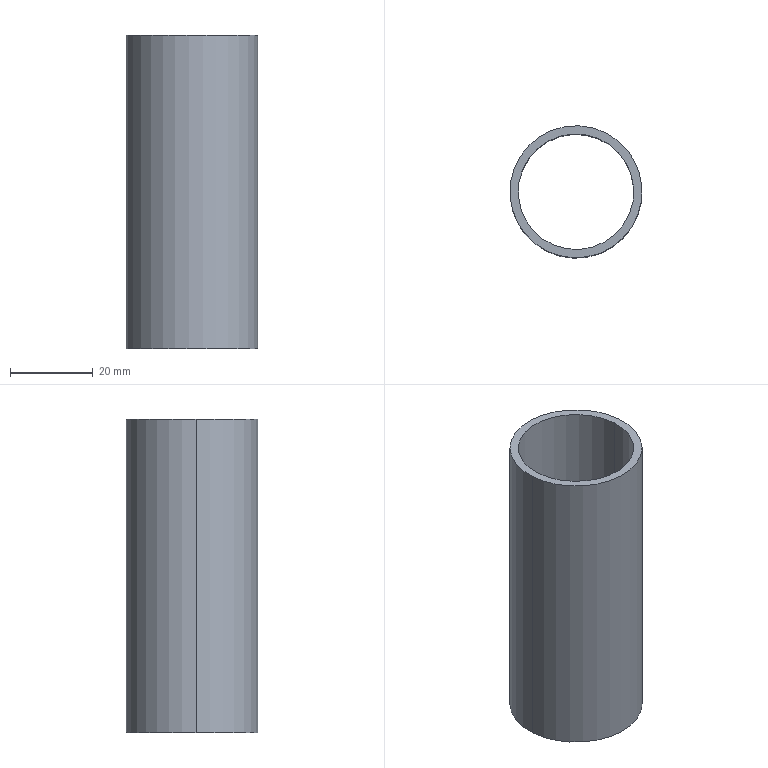Part | NX | features 0018 2 | 1 solid | 6 faces | box 32 x 32 x 76 mm | volume 14326 mm3 | cylinder 4 | plane 2 | commonest cylinder face diameters 28 x2 32 x2
STEP:
#1=CARTESIAN_POINT('',(-66.026,25.859,-286.129));
#2=VERTEX_POINT('',#1);
#3=CARTESIAN_POINT('',(-93.974,24.141,-286.129));
#4=VERTEX_POINT('',#3);
#5=CARTESIAN_POINT('',(-80.,25.,-286.129));
#6=DIRECTION('',(0.,0.,1.));
#7=DIRECTION('',(0.9981,0.06136,0.));
#8=AXIS2_PLACEMENT_3D('',#5,#6,#7);
#9=CIRCLE('',#8,14.);
#10=EDGE_CURVE('',#2,#4,#9,.T.);
#11=ORIENTED_EDGE('',*,*,#10,.F.);
#12=CARTESIAN_POINT('',(-66.026,25.859,-210.129));
#13=VERTEX_POINT('',#12);
#14=CARTESIAN_POINT('',(-66.026,25.859,-210.129));
#15=DIRECTION('',(0.,0.,-1.));
#16=VECTOR('',#15,1000.);
#17=LINE('',#14,#16);
#18=EDGE_CURVE('',#13,#2,#17,.T.);
#19=ORIENTED_EDGE('',*,*,#18,.F.);
#20=CARTESIAN_POINT('',(-93.974,24.141,-210.129));
#21=VERTEX_POINT('',#20);
#22=CARTESIAN_POINT('',(-80.,25.,-210.129));
#23=DIRECTION('',(0.,0.,-1.));
#24=DIRECTION('',(-0.9981,-0.06136,0.));
#25=AXIS2_PLACEMENT_3D('',#22,#23,#24);
#26=CIRCLE('',#25,14.);
#27=EDGE_CURVE('',#21,#13,#26,.T.);
#28=ORIENTED_EDGE('',*,*,#27,.F.);
#29=CARTESIAN_POINT('',(-93.974,24.141,-210.129));
#30=DIRECTION('',(0.,0.,-1.));
#31=VECTOR('',#30,1000.);
#32=LINE('',#29,#31);
#33=EDGE_CURVE('',#4,#21,#32,.F.);
#34=ORIENTED_EDGE('',*,*,#33,.F.);
#35=EDGE_LOOP('',(#11,#19,#28,#34));
#36=FACE_BOUND('',#35,.T.);
#37=CARTESIAN_POINT('',(-80.,25.,-286.129));
#38=DIRECTION('',(0.,0.,1.));
#39=DIRECTION('',(0.9981,0.06136,0.));
#40=AXIS2_PLACEMENT_3D('',#37,#38,#39);
#41=CYLINDRICAL_SURFACE('',#40,14.);
#42=ADVANCED_FACE('',(#36),#41,.F.);
#43=ORIENTED_EDGE('',*,*,#27,.T.);
#44=CARTESIAN_POINT('',(-80.,25.,-210.129));
#45=DIRECTION('',(0.,0.,-1.));
#46=DIRECTION('',(0.9981,0.06136,0.));
#47=AXIS2_PLACEMENT_3D('',#44,#45,#46);
#48=CIRCLE('',#47,14.);
#49=EDGE_CURVE('',#13,#21,#48,.T.);
#50=ORIENTED_EDGE('',*,*,#49,.T.);
#51=EDGE_LOOP('',(#43,#50));
#52=FACE_BOUND('',#51,.T.);
#53=CARTESIAN_POINT('',(-64.03,25.982,-210.129));
#54=VERTEX_POINT('',#53);
#55=CARTESIAN_POINT('',(-95.97,24.018,-210.129));
#56=VERTEX_POINT('',#55);
#57=CARTESIAN_POINT('',(-80.,25.,-210.129));
#58=DIRECTION('',(0.,0.,1.));
#59=DIRECTION('',(0.9981,0.06136,0.));
#60=AXIS2_PLACEMENT_3D('',#57,#58,#59);
#61=CIRCLE('',#60,16.);
#62=EDGE_CURVE('',#54,#56,#61,.T.);
#63=ORIENTED_EDGE('',*,*,#62,.T.);
#64=CARTESIAN_POINT('',(-80.,25.,-210.129));
#65=DIRECTION('',(0.,0.,1.));
#66=DIRECTION('',(-0.9981,-0.06136,0.));
#67=AXIS2_PLACEMENT_3D('',#64,#65,#66);
#68=CIRCLE('',#67,16.);
#69=EDGE_CURVE('',#56,#54,#68,.T.);
#70=ORIENTED_EDGE('',*,*,#69,.T.);
#71=EDGE_LOOP('',(#63,#70));
#72=FACE_BOUND('',#71,.T.);
#73=CARTESIAN_POINT('',(-80.,25.,-210.129));
#74=DIRECTION('',(0.,0.,-1.));
#75=DIRECTION('',(-0.9981,-0.06136,0.));
#76=AXIS2_PLACEMENT_3D('',#73,#74,#75);
#77=PLANE('',#76);
#78=ADVANCED_FACE('',(#52,#72),#77,.F.);
#79=CARTESIAN_POINT('',(-95.97,24.018,-286.129));
#80=VERTEX_POINT('',#79);
#81=CARTESIAN_POINT('',(-95.97,24.018,-210.129));
#82=DIRECTION('',(0.,0.,-1.));
#83=VECTOR('',#82,1000.);
#84=LINE('',#81,#83);
#85=EDGE_CURVE('',#56,#80,#84,.T.);
#86=ORIENTED_EDGE('',*,*,#85,.F.);
#87=ORIENTED_EDGE('',*,*,#62,.F.);
#88=CARTESIAN_POINT('',(-64.03,25.982,-286.129));
#89=VERTEX_POINT('',#88);
#90=CARTESIAN_POINT('',(-64.03,25.982,-210.129));
#91=DIRECTION('',(0.,0.,-1.));
#92=VECTOR('',#91,1000.);
#93=LINE('',#90,#92);
#94=EDGE_CURVE('',#89,#54,#93,.F.);
#95=ORIENTED_EDGE('',*,*,#94,.F.);
#96=CARTESIAN_POINT('',(-80.,25.,-286.129));
#97=DIRECTION('',(0.,0.,-1.));
#98=DIRECTION('',(-0.9981,-0.06136,0.));
#99=AXIS2_PLACEMENT_3D('',#96,#97,#98);
#100=CIRCLE('',#99,16.);
#101=EDGE_CURVE('',#80,#89,#100,.T.);
#102=ORIENTED_EDGE('',*,*,#101,.F.);
#103=EDGE_LOOP('',(#86,#87,#95,#102));
#104=FACE_BOUND('',#103,.T.);
#105=CARTESIAN_POINT('',(-80.,25.,-286.129));
#106=DIRECTION('',(0.,0.,1.));
#107=DIRECTION('',(0.9981,0.06136,0.));
#108=AXIS2_PLACEMENT_3D('',#105,#106,#107);
#109=CYLINDRICAL_SURFACE('',#108,16.);
#110=ADVANCED_FACE('',(#104),#109,.T.);
#111=CARTESIAN_POINT('',(-80.,25.,-286.129));
#112=DIRECTION('',(0.,0.,-1.));
#113=DIRECTION('',(0.9981,0.06136,0.));
#114=AXIS2_PLACEMENT_3D('',#111,#112,#113);
#115=CIRCLE('',#114,16.);
#116=EDGE_CURVE('',#89,#80,#115,.T.);
#117=ORIENTED_EDGE('',*,*,#116,.F.);
#118=ORIENTED_EDGE('',*,*,#94,.T.);
#119=ORIENTED_EDGE('',*,*,#69,.F.);
#120=ORIENTED_EDGE('',*,*,#85,.T.);
#121=EDGE_LOOP('',(#117,#118,#119,#120));
#122=FACE_BOUND('',#121,.T.);
#123=CARTESIAN_POINT('',(-80.,25.,-286.129));
#124=DIRECTION('',(0.,0.,1.));
#125=DIRECTION('',(0.9981,0.06136,0.));
#126=AXIS2_PLACEMENT_3D('',#123,#124,#125);
#127=CYLINDRICAL_SURFACE('',#126,16.);
#128=ADVANCED_FACE('',(#122),#127,.T.);
#129=ORIENTED_EDGE('',*,*,#10,.T.);
#130=CARTESIAN_POINT('',(-80.,25.,-286.129));
#131=DIRECTION('',(0.,0.,1.));
#132=DIRECTION('',(-0.9981,-0.06136,0.));
#133=AXIS2_PLACEMENT_3D('',#130,#131,#132);
#134=CIRCLE('',#133,14.);
#135=EDGE_CURVE('',#4,#2,#134,.T.);
#136=ORIENTED_EDGE('',*,*,#135,.T.);
#137=EDGE_LOOP('',(#129,#136));
#138=FACE_BOUND('',#137,.T.);
#139=ORIENTED_EDGE('',*,*,#101,.T.);
#140=ORIENTED_EDGE('',*,*,#116,.T.);
#141=EDGE_LOOP('',(#139,#140));
#142=FACE_BOUND('',#141,.T.);
#143=CARTESIAN_POINT('',(-80.,25.,-286.129));
#144=DIRECTION('',(0.,0.,-1.));
#145=DIRECTION('',(-0.9981,-0.06136,0.));
#146=AXIS2_PLACEMENT_3D('',#143,#144,#145);
#147=PLANE('',#146);
#148=ADVANCED_FACE('',(#138,#142),#147,.T.);
#149=ORIENTED_EDGE('',*,*,#33,.T.);
#150=ORIENTED_EDGE('',*,*,#49,.F.);
#151=ORIENTED_EDGE('',*,*,#18,.T.);
#152=ORIENTED_EDGE('',*,*,#135,.F.);
#153=EDGE_LOOP('',(#149,#150,#151,#152));
#154=FACE_BOUND('',#153,.T.);
#155=CARTESIAN_POINT('',(-80.,25.,-286.129));
#156=DIRECTION('',(0.,0.,1.));
#157=DIRECTION('',(0.9981,0.06136,0.));
#158=AXIS2_PLACEMENT_3D('',#155,#156,#157);
#159=CYLINDRICAL_SURFACE('',#158,14.);
#160=ADVANCED_FACE('',(#154),#159,.F.);
#161=CLOSED_SHELL('',(#42,#78,#110,#128,#148,#160));
#162=MANIFOLD_SOLID_BREP('',#161);
#163=(LENGTH_UNIT()NAMED_UNIT(*)SI_UNIT(.MILLI.,.METRE.));
#164=UNCERTAINTY_MEASURE_WITH_UNIT(LENGTH_MEASURE(0.00001),#163,'','');
#165=(NAMED_UNIT(*)PLANE_ANGLE_UNIT()SI_UNIT($,.RADIAN.));
#166=(NAMED_UNIT(*)SI_UNIT($,.STERADIAN.)SOLID_ANGLE_UNIT());
#167=(GEOMETRIC_REPRESENTATION_CONTEXT(3)GLOBAL_UNCERTAINTY_ASSIGNED_CONTEXT((#164))GLOBAL_UNIT_ASSIGNED_CONTEXT((#163,#165,#166))REPRESENTATION_CONTEXT('',''));
#168=ADVANCED_BREP_SHAPE_REPRESENTATION('',(#162),#167);